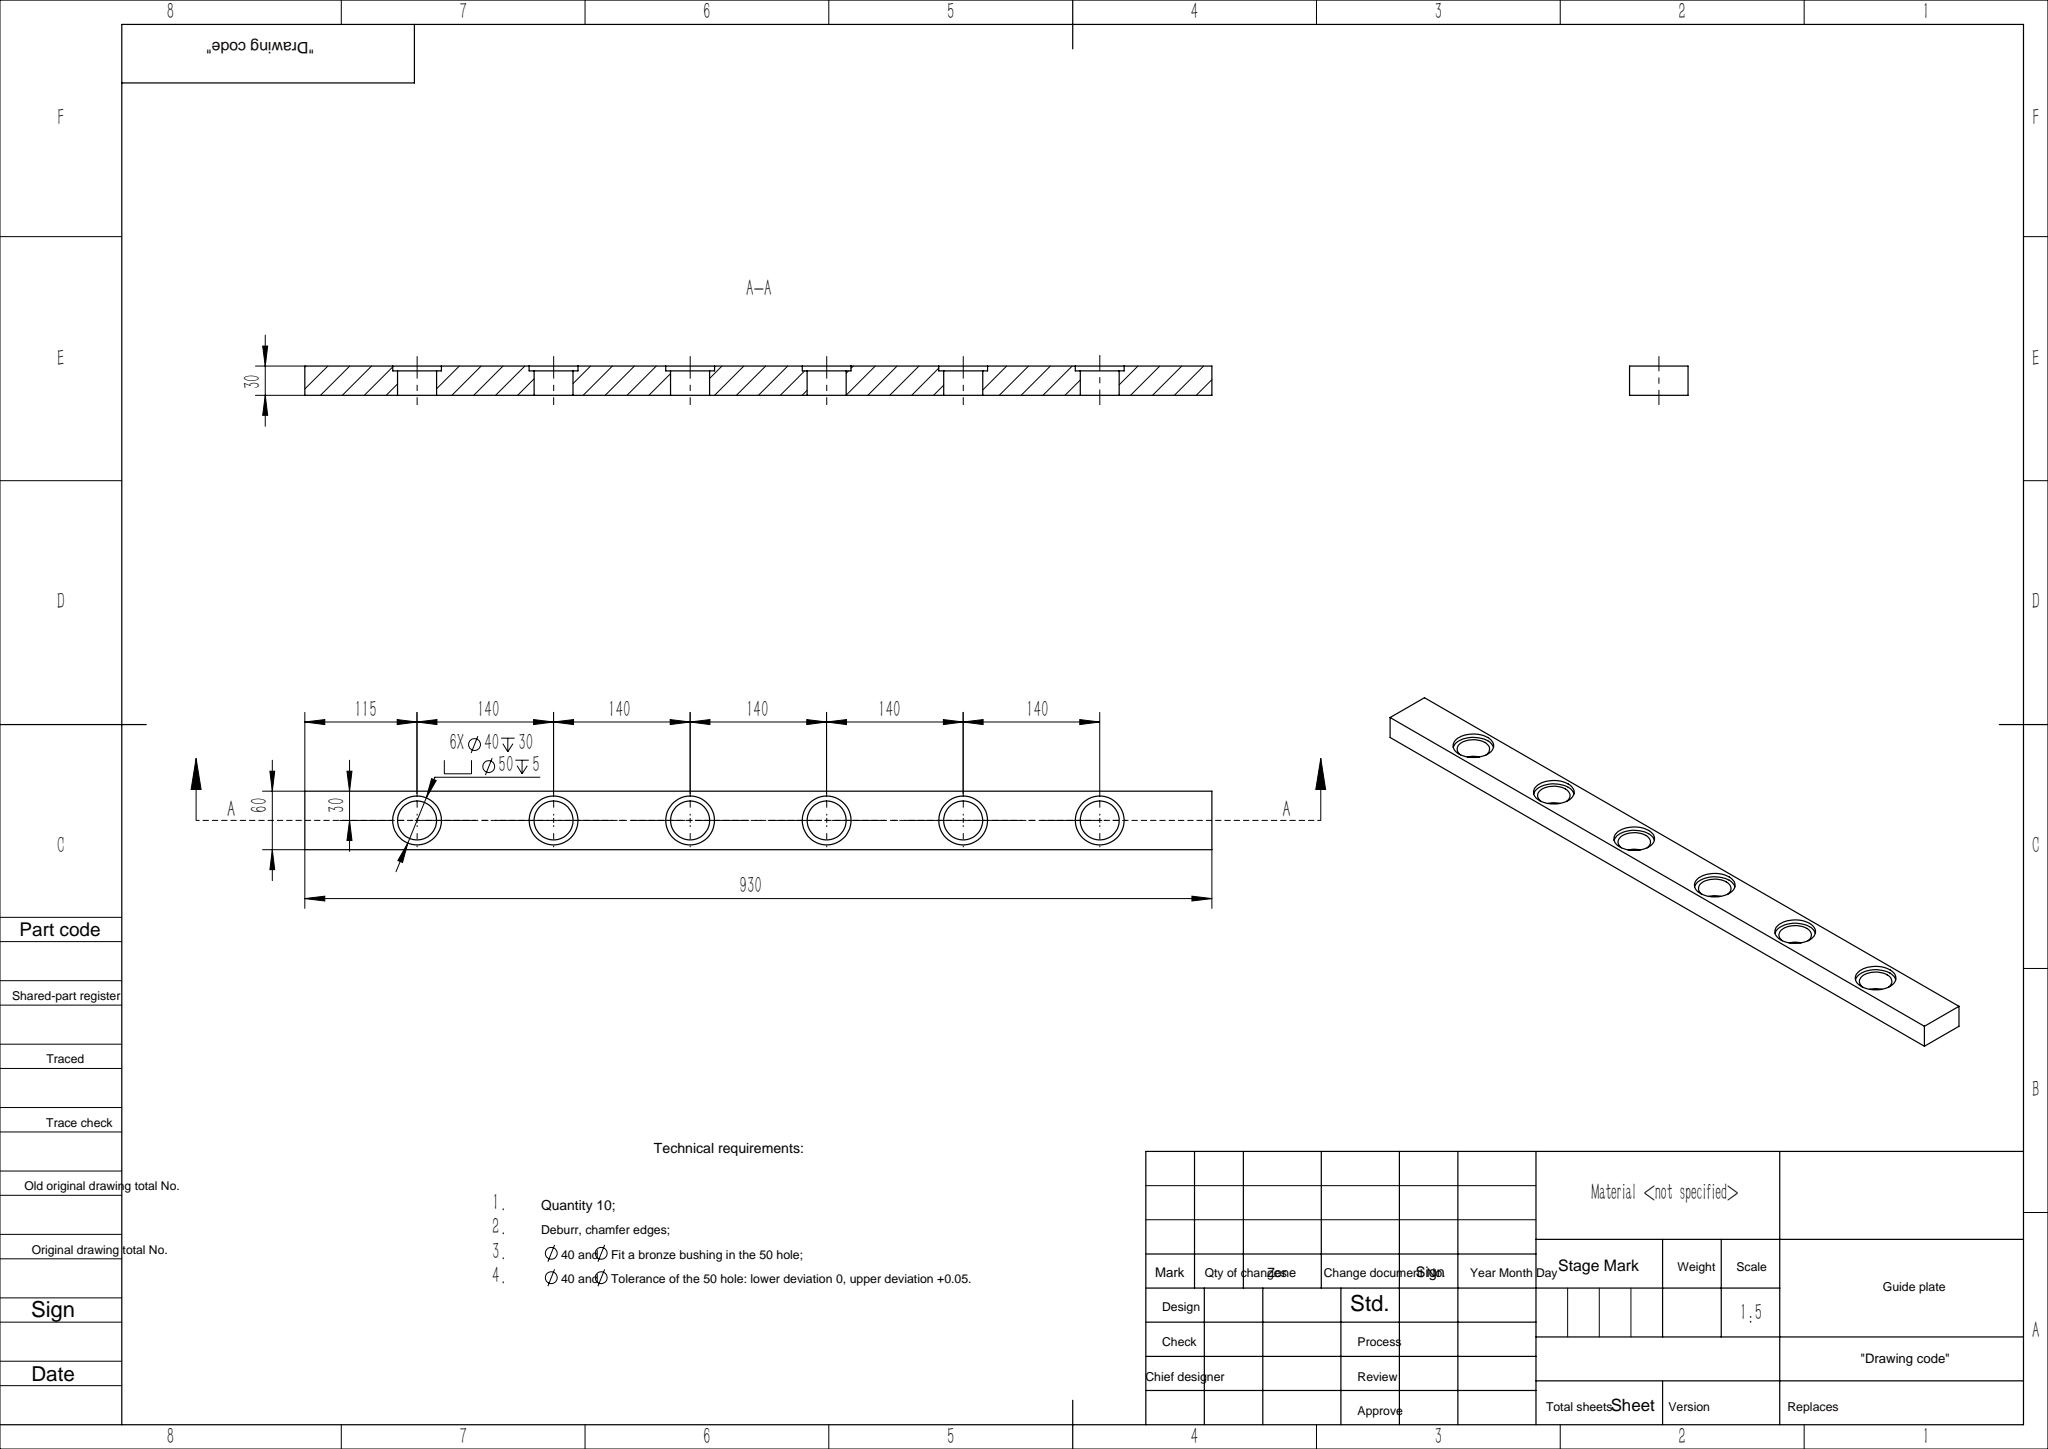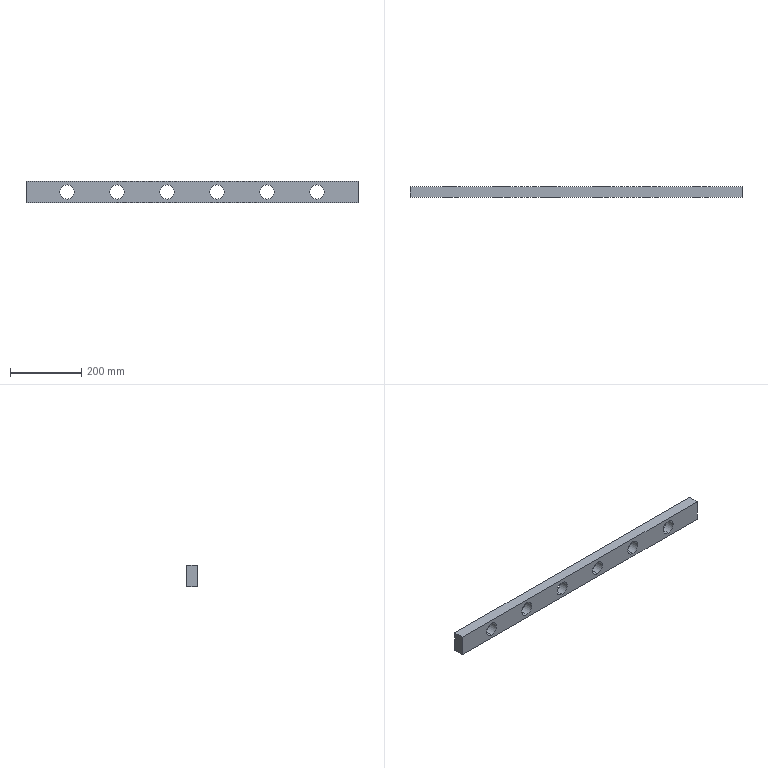Part | SolidWorks | features Extrusion 1, LPattern 1, RevCut 1 | 1 solid | 36 faces | box 930 x 30 x 60 mm | volume 1426600 mm3 | cylinder 24 | plane 12 | commonest cylinder face diameters 40 x12 50 x12